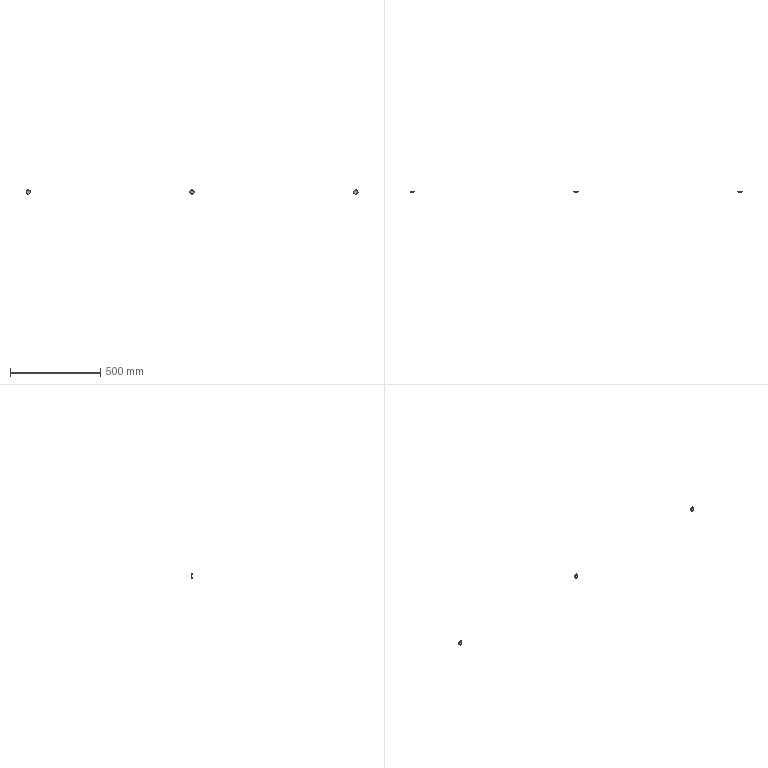Part | STEP file | DCV-000-W09-2300L_1 | 6 solids | 24 faces | box 1844 x 5.469 x 24 mm | volume 1672 mm3 | cylinder 18 | plane 6 | commonest cylinder face diameters 24 x12 31.8 x6